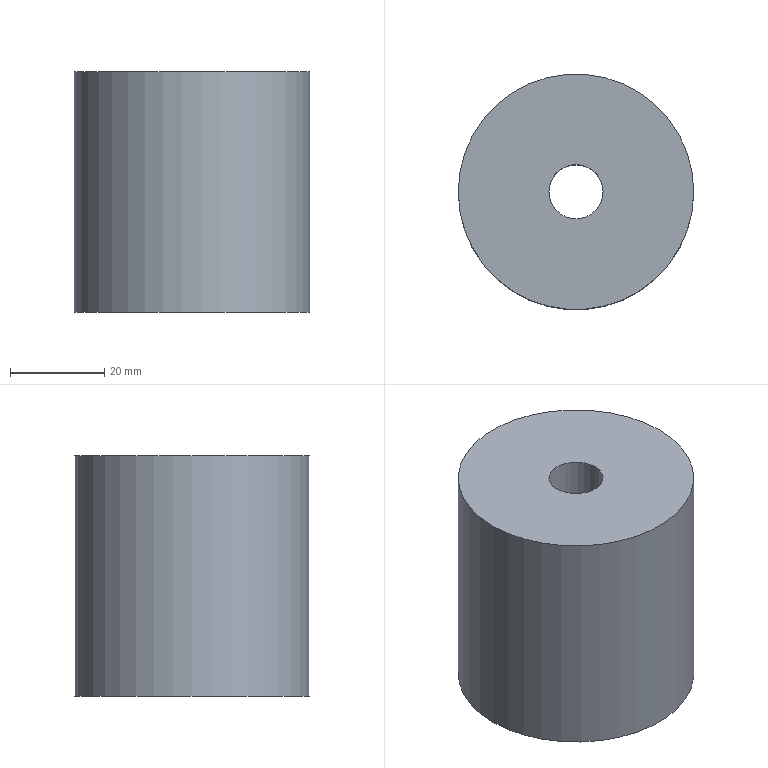Part | NX | features 9 2 | 1 solid | 6 faces | box 50 x 50 x 51 mm | volume 92130 mm3 | cylinder 3 | plane 3 | commonest cylinder face diameters 11.5 x1 18 x1 50 x1
STEP:
#1=CARTESIAN_POINT('',(-23.,560.,50.));
#2=VERTEX_POINT('',#1);
#3=CARTESIAN_POINT('',(2.,560.,50.));
#4=DIRECTION('',(0.,0.,1.));
#5=DIRECTION('',(-1.,0.,0.));
#6=AXIS2_PLACEMENT_3D('',#3,#4,#5);
#7=CIRCLE('',#6,25.);
#8=EDGE_CURVE('',#2,#2,#7,.T.);
#9=ORIENTED_EDGE('',*,*,#8,.T.);
#10=EDGE_LOOP('',(#9));
#11=FACE_BOUND('',#10,.T.);
#12=CARTESIAN_POINT('',(-23.,560.,101.));
#13=VERTEX_POINT('',#12);
#14=CARTESIAN_POINT('',(2.,560.,101.));
#15=DIRECTION('',(0.,0.,-1.));
#16=DIRECTION('',(-1.,0.,0.));
#17=AXIS2_PLACEMENT_3D('',#14,#15,#16);
#18=CIRCLE('',#17,25.);
#19=EDGE_CURVE('',#13,#13,#18,.T.);
#20=ORIENTED_EDGE('',*,*,#19,.T.);
#21=EDGE_LOOP('',(#20));
#22=FACE_BOUND('',#21,.T.);
#23=CARTESIAN_POINT('',(2.,560.,20.));
#24=DIRECTION('',(0.,0.,-1.));
#25=DIRECTION('',(-1.,0.,0.));
#26=AXIS2_PLACEMENT_3D('',#23,#24,#25);
#27=CYLINDRICAL_SURFACE('',#26,25.);
#28=ADVANCED_FACE('',(#11,#22),#27,.T.);
#29=CARTESIAN_POINT('',(7.75,560.,68.));
#30=VERTEX_POINT('',#29);
#31=CARTESIAN_POINT('',(2.,560.,68.));
#32=DIRECTION('',(0.,0.,1.));
#33=DIRECTION('',(1.,0.,0.));
#34=AXIS2_PLACEMENT_3D('',#31,#32,#33);
#35=CIRCLE('',#34,5.75);
#36=EDGE_CURVE('',#30,#30,#35,.T.);
#37=ORIENTED_EDGE('',*,*,#36,.F.);
#38=EDGE_LOOP('',(#37));
#39=FACE_BOUND('',#38,.T.);
#40=CARTESIAN_POINT('',(7.75,560.,101.));
#41=VERTEX_POINT('',#40);
#42=CARTESIAN_POINT('',(2.,560.,101.));
#43=DIRECTION('',(0.,0.,1.));
#44=DIRECTION('',(1.,0.,0.));
#45=AXIS2_PLACEMENT_3D('',#42,#43,#44);
#46=CIRCLE('',#45,5.75);
#47=EDGE_CURVE('',#41,#41,#46,.T.);
#48=ORIENTED_EDGE('',*,*,#47,.T.);
#49=EDGE_LOOP('',(#48));
#50=FACE_BOUND('',#49,.T.);
#51=CARTESIAN_POINT('',(2.,560.,55.));
#52=DIRECTION('',(0.,0.,1.));
#53=DIRECTION('',(1.,0.,0.));
#54=AXIS2_PLACEMENT_3D('',#51,#52,#53);
#55=CYLINDRICAL_SURFACE('',#54,5.75);
#56=ADVANCED_FACE('',(#39,#50),#55,.F.);
#57=CARTESIAN_POINT('',(-7.,560.,68.));
#58=VERTEX_POINT('',#57);
#59=CARTESIAN_POINT('',(2.,560.,68.));
#60=DIRECTION('',(0.,0.,1.));
#61=DIRECTION('',(-1.,0.,0.));
#62=AXIS2_PLACEMENT_3D('',#59,#60,#61);
#63=CIRCLE('',#62,9.);
#64=EDGE_CURVE('',#58,#58,#63,.T.);
#65=ORIENTED_EDGE('',*,*,#64,.T.);
#66=EDGE_LOOP('',(#65));
#67=FACE_BOUND('',#66,.T.);
#68=CARTESIAN_POINT('',(11.,560.,50.));
#69=VERTEX_POINT('',#68);
#70=CARTESIAN_POINT('',(2.,560.,50.));
#71=DIRECTION('',(0.,0.,-1.));
#72=DIRECTION('',(1.,0.,0.));
#73=AXIS2_PLACEMENT_3D('',#70,#71,#72);
#74=CIRCLE('',#73,9.);
#75=EDGE_CURVE('',#69,#69,#74,.T.);
#76=ORIENTED_EDGE('',*,*,#75,.T.);
#77=EDGE_LOOP('',(#76));
#78=FACE_BOUND('',#77,.T.);
#79=CARTESIAN_POINT('',(2.,560.,20.));
#80=DIRECTION('',(0.,0.,1.));
#81=DIRECTION('',(1.,0.,0.));
#82=AXIS2_PLACEMENT_3D('',#79,#80,#81);
#83=CYLINDRICAL_SURFACE('',#82,9.);
#84=ADVANCED_FACE('',(#67,#78),#83,.F.);
#85=ORIENTED_EDGE('',*,*,#36,.T.);
#86=EDGE_LOOP('',(#85));
#87=FACE_BOUND('',#86,.T.);
#88=ORIENTED_EDGE('',*,*,#64,.F.);
#89=EDGE_LOOP('',(#88));
#90=FACE_BOUND('',#89,.T.);
#91=CARTESIAN_POINT('',(2.,560.,68.));
#92=DIRECTION('',(0.,0.,1.));
#93=DIRECTION('',(1.,0.,0.));
#94=AXIS2_PLACEMENT_3D('',#91,#92,#93);
#95=PLANE('',#94);
#96=ADVANCED_FACE('',(#87,#90),#95,.F.);
#97=ORIENTED_EDGE('',*,*,#75,.F.);
#98=EDGE_LOOP('',(#97));
#99=FACE_BOUND('',#98,.T.);
#100=ORIENTED_EDGE('',*,*,#8,.F.);
#101=EDGE_LOOP('',(#100));
#102=FACE_BOUND('',#101,.T.);
#103=CARTESIAN_POINT('',(340.,815.,50.));
#104=DIRECTION('',(0.,0.,-1.));
#105=DIRECTION('',(-1.,0.,0.));
#106=AXIS2_PLACEMENT_3D('',#103,#104,#105);
#107=PLANE('',#106);
#108=ADVANCED_FACE('',(#99,#102),#107,.T.);
#109=ORIENTED_EDGE('',*,*,#47,.F.);
#110=EDGE_LOOP('',(#109));
#111=FACE_BOUND('',#110,.T.);
#112=ORIENTED_EDGE('',*,*,#19,.F.);
#113=EDGE_LOOP('',(#112));
#114=FACE_BOUND('',#113,.T.);
#115=CARTESIAN_POINT('',(-490.,939.,101.));
#116=DIRECTION('',(0.,0.,1.));
#117=DIRECTION('',(-1.,0.,0.));
#118=AXIS2_PLACEMENT_3D('',#115,#116,#117);
#119=PLANE('',#118);
#120=ADVANCED_FACE('',(#111,#114),#119,.T.);
#121=CLOSED_SHELL('',(#28,#56,#84,#96,#108,#120));
#122=MANIFOLD_SOLID_BREP('',#121);
#123=(LENGTH_UNIT()NAMED_UNIT(*)SI_UNIT(.MILLI.,.METRE.));
#124=UNCERTAINTY_MEASURE_WITH_UNIT(LENGTH_MEASURE(0.00001),#123,'','');
#125=(NAMED_UNIT(*)PLANE_ANGLE_UNIT()SI_UNIT($,.RADIAN.));
#126=(NAMED_UNIT(*)SI_UNIT($,.STERADIAN.)SOLID_ANGLE_UNIT());
#127=(GEOMETRIC_REPRESENTATION_CONTEXT(3)GLOBAL_UNCERTAINTY_ASSIGNED_CONTEXT((#124))GLOBAL_UNIT_ASSIGNED_CONTEXT((#123,#125,#126))REPRESENTATION_CONTEXT('',''));
#128=ADVANCED_BREP_SHAPE_REPRESENTATION('',(#122),#127);